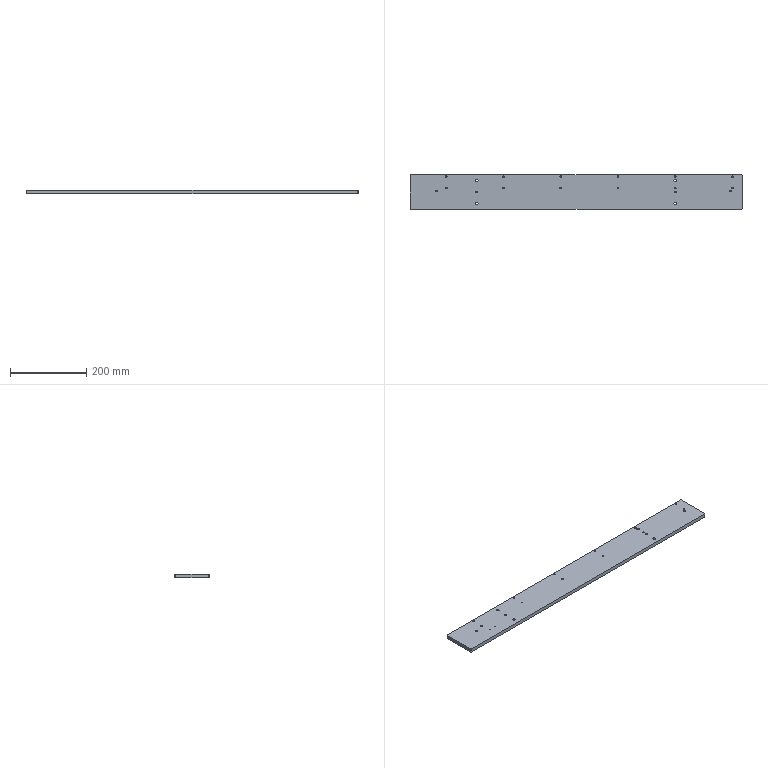Part | SolidWorks | features HoleWzd 4, Chamfer 1, Extrusion 1, ICE 1, LPattern 1 | 1 solid | 78 faces | box 870 x 90 x 10 mm | volume 777394 mm3 | cylinder 56 | plane 14 | cone 8 | commonest cylinder face diameters 4.2 x24 2.5 x8 5 x8 6.6 x8 11 x8